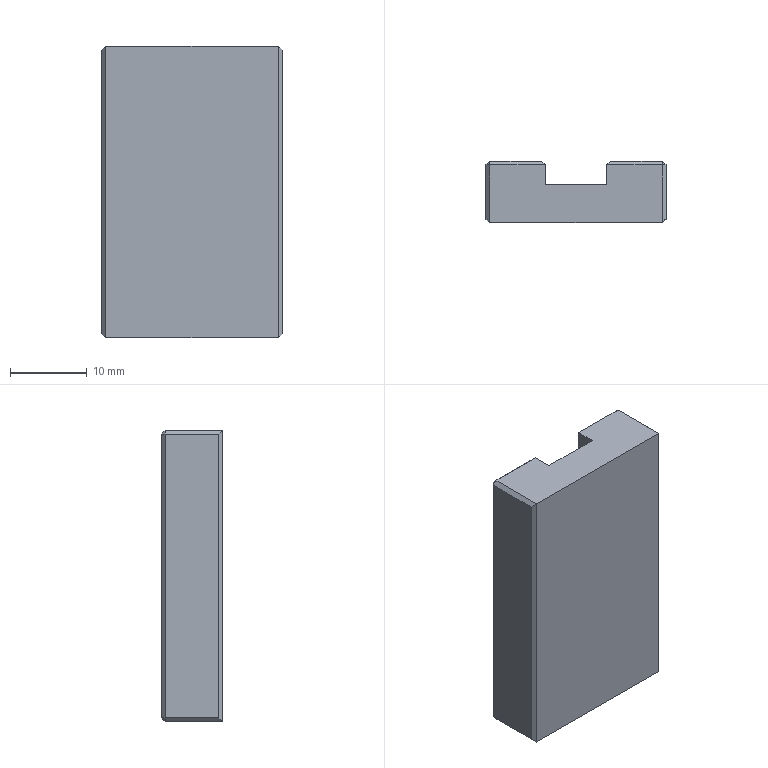Part | SolidWorks | features Chamfer 1, Extrusion 1 | 1 solid | 28 faces | box 23.5 x 8 x 38 mm | volume 6196 mm3 | plane 28
STEP:
#1=CARTESIAN_POINT('',(11.75,3.5,37.5));
#2=VERTEX_POINT('',#1);
#3=CARTESIAN_POINT('',(11.75,-3.5,37.5));
#4=VERTEX_POINT('',#3);
#5=CARTESIAN_POINT('',(11.75,-4.,37.5));
#6=DIRECTION('',(0.,-1.,0.));
#7=VECTOR('',#6,1000.);
#8=LINE('',#5,#7);
#9=EDGE_CURVE('',#2,#4,#8,.T.);
#10=ORIENTED_EDGE('',*,*,#9,.T.);
#11=CARTESIAN_POINT('',(11.75,-3.5,0.5));
#12=VERTEX_POINT('',#11);
#13=CARTESIAN_POINT('',(11.75,-3.5,38.));
#14=DIRECTION('',(0.,0.,-1.));
#15=VECTOR('',#14,1000.);
#16=LINE('',#13,#15);
#17=EDGE_CURVE('',#4,#12,#16,.T.);
#18=ORIENTED_EDGE('',*,*,#17,.T.);
#19=CARTESIAN_POINT('',(11.75,3.5,0.5));
#20=VERTEX_POINT('',#19);
#21=CARTESIAN_POINT('',(11.75,4.,0.5));
#22=DIRECTION('',(0.,1.,0.));
#23=VECTOR('',#22,1000.);
#24=LINE('',#21,#23);
#25=EDGE_CURVE('',#12,#20,#24,.T.);
#26=ORIENTED_EDGE('',*,*,#25,.T.);
#27=CARTESIAN_POINT('',(11.75,3.5,38.));
#28=DIRECTION('',(0.,0.,1.));
#29=VECTOR('',#28,1000.);
#30=LINE('',#27,#29);
#31=EDGE_CURVE('',#20,#2,#30,.T.);
#32=ORIENTED_EDGE('',*,*,#31,.T.);
#33=EDGE_LOOP('',(#10,#18,#26,#32));
#34=FACE_OUTER_BOUND('',#33,.T.);
#35=CARTESIAN_POINT('',(11.75,4.,38.));
#36=DIRECTION('',(-1.,0.,0.));
#37=DIRECTION('',(0.,-1.,0.));
#38=AXIS2_PLACEMENT_3D('',#35,#36,#37);
#39=PLANE('',#38);
#40=ADVANCED_FACE('',(#34),#39,.F.);
#41=CARTESIAN_POINT('',(4.5,4.,37.5));
#42=VERTEX_POINT('',#41);
#43=CARTESIAN_POINT('',(11.25,4.,37.5));
#44=VERTEX_POINT('',#43);
#45=CARTESIAN_POINT('',(11.75,4.,37.5));
#46=DIRECTION('',(1.,0.,0.));
#47=VECTOR('',#46,1000.);
#48=LINE('',#45,#47);
#49=EDGE_CURVE('',#42,#44,#48,.T.);
#50=ORIENTED_EDGE('',*,*,#49,.T.);
#51=CARTESIAN_POINT('',(11.25,4.,0.5));
#52=VERTEX_POINT('',#51);
#53=CARTESIAN_POINT('',(11.25,4.,38.));
#54=DIRECTION('',(0.,0.,-1.));
#55=VECTOR('',#54,1000.);
#56=LINE('',#53,#55);
#57=EDGE_CURVE('',#44,#52,#56,.T.);
#58=ORIENTED_EDGE('',*,*,#57,.T.);
#59=CARTESIAN_POINT('',(4.5,4.,0.5));
#60=VERTEX_POINT('',#59);
#61=CARTESIAN_POINT('',(4.,4.,0.5));
#62=DIRECTION('',(-1.,0.,0.));
#63=VECTOR('',#62,1000.);
#64=LINE('',#61,#63);
#65=EDGE_CURVE('',#52,#60,#64,.T.);
#66=ORIENTED_EDGE('',*,*,#65,.T.);
#67=CARTESIAN_POINT('',(4.5,4.,38.));
#68=DIRECTION('',(0.,0.,1.));
#69=VECTOR('',#68,1000.);
#70=LINE('',#67,#69);
#71=EDGE_CURVE('',#60,#42,#70,.T.);
#72=ORIENTED_EDGE('',*,*,#71,.T.);
#73=EDGE_LOOP('',(#50,#58,#66,#72));
#74=FACE_OUTER_BOUND('',#73,.T.);
#75=CARTESIAN_POINT('',(4.,4.,38.));
#76=DIRECTION('',(0.,-1.,0.));
#77=DIRECTION('',(1.,0.,0.));
#78=AXIS2_PLACEMENT_3D('',#75,#76,#77);
#79=PLANE('',#78);
#80=ADVANCED_FACE('',(#74),#79,.F.);
#81=CARTESIAN_POINT('',(4.,3.5,38.));
#82=VERTEX_POINT('',#81);
#83=CARTESIAN_POINT('',(4.,1.,38.));
#84=VERTEX_POINT('',#83);
#85=CARTESIAN_POINT('',(4.,1.,38.));
#86=DIRECTION('',(0.,-1.,0.));
#87=VECTOR('',#86,1000.);
#88=LINE('',#85,#87);
#89=EDGE_CURVE('',#82,#84,#88,.T.);
#90=ORIENTED_EDGE('',*,*,#89,.F.);
#91=CARTESIAN_POINT('',(4.,3.5,0.));
#92=VERTEX_POINT('',#91);
#93=CARTESIAN_POINT('',(4.,3.5,38.));
#94=DIRECTION('',(0.,0.,-1.));
#95=VECTOR('',#94,1000.);
#96=LINE('',#93,#95);
#97=EDGE_CURVE('',#82,#92,#96,.T.);
#98=ORIENTED_EDGE('',*,*,#97,.T.);
#99=CARTESIAN_POINT('',(4.,1.,0.));
#100=VERTEX_POINT('',#99);
#101=CARTESIAN_POINT('',(4.,1.,0.));
#102=DIRECTION('',(0.,-1.,0.));
#103=VECTOR('',#102,1000.);
#104=LINE('',#101,#103);
#105=EDGE_CURVE('',#92,#100,#104,.T.);
#106=ORIENTED_EDGE('',*,*,#105,.T.);
#107=CARTESIAN_POINT('',(4.,1.,38.));
#108=DIRECTION('',(0.,0.,-1.));
#109=VECTOR('',#108,1000.);
#110=LINE('',#107,#109);
#111=EDGE_CURVE('',#84,#100,#110,.T.);
#112=ORIENTED_EDGE('',*,*,#111,.F.);
#113=EDGE_LOOP('',(#90,#98,#106,#112));
#114=FACE_OUTER_BOUND('',#113,.T.);
#115=CARTESIAN_POINT('',(4.,1.,38.));
#116=DIRECTION('',(1.,0.,0.));
#117=DIRECTION('',(0.,1.,0.));
#118=AXIS2_PLACEMENT_3D('',#115,#116,#117);
#119=PLANE('',#118);
#120=ADVANCED_FACE('',(#114),#119,.F.);
#121=CARTESIAN_POINT('',(-4.,1.,0.));
#122=VERTEX_POINT('',#121);
#123=CARTESIAN_POINT('',(-4.,1.,0.));
#124=DIRECTION('',(-1.,0.,0.));
#125=VECTOR('',#124,1000.);
#126=LINE('',#123,#125);
#127=EDGE_CURVE('',#100,#122,#126,.T.);
#128=ORIENTED_EDGE('',*,*,#127,.T.);
#129=CARTESIAN_POINT('',(-4.,1.,38.));
#130=VERTEX_POINT('',#129);
#131=CARTESIAN_POINT('',(-4.,1.,38.));
#132=DIRECTION('',(0.,0.,-1.));
#133=VECTOR('',#132,1000.);
#134=LINE('',#131,#133);
#135=EDGE_CURVE('',#130,#122,#134,.T.);
#136=ORIENTED_EDGE('',*,*,#135,.F.);
#137=CARTESIAN_POINT('',(-4.,1.,38.));
#138=DIRECTION('',(-1.,0.,0.));
#139=VECTOR('',#138,1000.);
#140=LINE('',#137,#139);
#141=EDGE_CURVE('',#84,#130,#140,.T.);
#142=ORIENTED_EDGE('',*,*,#141,.F.);
#143=ORIENTED_EDGE('',*,*,#111,.T.);
#144=EDGE_LOOP('',(#128,#136,#142,#143));
#145=FACE_OUTER_BOUND('',#144,.T.);
#146=CARTESIAN_POINT('',(-4.,1.,38.));
#147=DIRECTION('',(0.,-1.,0.));
#148=DIRECTION('',(1.,0.,0.));
#149=AXIS2_PLACEMENT_3D('',#146,#147,#148);
#150=PLANE('',#149);
#151=ADVANCED_FACE('',(#145),#150,.F.);
#152=CARTESIAN_POINT('',(-4.,3.5,0.));
#153=VERTEX_POINT('',#152);
#154=CARTESIAN_POINT('',(-4.,4.,0.));
#155=DIRECTION('',(0.,1.,0.));
#156=VECTOR('',#155,1000.);
#157=LINE('',#154,#156);
#158=EDGE_CURVE('',#122,#153,#157,.T.);
#159=ORIENTED_EDGE('',*,*,#158,.T.);
#160=CARTESIAN_POINT('',(-4.,3.5,38.));
#161=VERTEX_POINT('',#160);
#162=CARTESIAN_POINT('',(-4.,3.5,38.));
#163=DIRECTION('',(0.,0.,1.));
#164=VECTOR('',#163,1000.);
#165=LINE('',#162,#164);
#166=EDGE_CURVE('',#153,#161,#165,.T.);
#167=ORIENTED_EDGE('',*,*,#166,.T.);
#168=CARTESIAN_POINT('',(-4.,4.,38.));
#169=DIRECTION('',(0.,1.,0.));
#170=VECTOR('',#169,1000.);
#171=LINE('',#168,#170);
#172=EDGE_CURVE('',#130,#161,#171,.T.);
#173=ORIENTED_EDGE('',*,*,#172,.F.);
#174=ORIENTED_EDGE('',*,*,#135,.T.);
#175=EDGE_LOOP('',(#159,#167,#173,#174));
#176=FACE_OUTER_BOUND('',#175,.T.);
#177=CARTESIAN_POINT('',(-4.,4.,38.));
#178=DIRECTION('',(-1.,0.,0.));
#179=DIRECTION('',(0.,0.,1.));
#180=AXIS2_PLACEMENT_3D('',#177,#178,#179);
#181=PLANE('',#180);
#182=ADVANCED_FACE('',(#176),#181,.F.);
#183=CARTESIAN_POINT('',(-11.25,4.,37.5));
#184=VERTEX_POINT('',#183);
#185=CARTESIAN_POINT('',(-4.5,4.,37.5));
#186=VERTEX_POINT('',#185);
#187=CARTESIAN_POINT('',(-4.,4.,37.5));
#188=DIRECTION('',(1.,0.,0.));
#189=VECTOR('',#188,1000.);
#190=LINE('',#187,#189);
#191=EDGE_CURVE('',#184,#186,#190,.T.);
#192=ORIENTED_EDGE('',*,*,#191,.T.);
#193=CARTESIAN_POINT('',(-4.5,4.,0.5));
#194=VERTEX_POINT('',#193);
#195=CARTESIAN_POINT('',(-4.5,4.,38.));
#196=DIRECTION('',(0.,0.,-1.));
#197=VECTOR('',#196,1000.);
#198=LINE('',#195,#197);
#199=EDGE_CURVE('',#186,#194,#198,.T.);
#200=ORIENTED_EDGE('',*,*,#199,.T.);
#201=CARTESIAN_POINT('',(-11.25,4.,0.5));
#202=VERTEX_POINT('',#201);
#203=CARTESIAN_POINT('',(-11.75,4.,0.5));
#204=DIRECTION('',(-1.,0.,0.));
#205=VECTOR('',#204,1000.);
#206=LINE('',#203,#205);
#207=EDGE_CURVE('',#194,#202,#206,.T.);
#208=ORIENTED_EDGE('',*,*,#207,.T.);
#209=CARTESIAN_POINT('',(-11.25,4.,38.));
#210=DIRECTION('',(0.,0.,1.));
#211=VECTOR('',#210,1000.);
#212=LINE('',#209,#211);
#213=EDGE_CURVE('',#202,#184,#212,.T.);
#214=ORIENTED_EDGE('',*,*,#213,.T.);
#215=EDGE_LOOP('',(#192,#200,#208,#214));
#216=FACE_OUTER_BOUND('',#215,.T.);
#217=CARTESIAN_POINT('',(-11.75,4.,38.));
#218=DIRECTION('',(0.,-1.,0.));
#219=DIRECTION('',(0.,0.,-1.));
#220=AXIS2_PLACEMENT_3D('',#217,#218,#219);
#221=PLANE('',#220);
#222=ADVANCED_FACE('',(#216),#221,.F.);
#223=CARTESIAN_POINT('',(-11.75,-3.5,0.5));
#224=VERTEX_POINT('',#223);
#225=CARTESIAN_POINT('',(-11.75,-3.5,37.5));
#226=VERTEX_POINT('',#225);
#227=CARTESIAN_POINT('',(-11.75,-3.5,38.));
#228=DIRECTION('',(0.,0.,1.));
#229=VECTOR('',#228,1000.);
#230=LINE('',#227,#229);
#231=EDGE_CURVE('',#224,#226,#230,.T.);
#232=ORIENTED_EDGE('',*,*,#231,.T.);
#233=CARTESIAN_POINT('',(-11.75,3.5,37.5));
#234=VERTEX_POINT('',#233);
#235=CARTESIAN_POINT('',(-11.75,4.,37.5));
#236=DIRECTION('',(0.,1.,0.));
#237=VECTOR('',#236,1000.);
#238=LINE('',#235,#237);
#239=EDGE_CURVE('',#226,#234,#238,.T.);
#240=ORIENTED_EDGE('',*,*,#239,.T.);
#241=CARTESIAN_POINT('',(-11.75,3.5,0.5));
#242=VERTEX_POINT('',#241);
#243=CARTESIAN_POINT('',(-11.75,3.5,38.));
#244=DIRECTION('',(0.,0.,-1.));
#245=VECTOR('',#244,1000.);
#246=LINE('',#243,#245);
#247=EDGE_CURVE('',#234,#242,#246,.T.);
#248=ORIENTED_EDGE('',*,*,#247,.T.);
#249=CARTESIAN_POINT('',(-11.75,4.,0.5));
#250=DIRECTION('',(0.,-1.,0.));
#251=VECTOR('',#250,1000.);
#252=LINE('',#249,#251);
#253=EDGE_CURVE('',#242,#224,#252,.T.);
#254=ORIENTED_EDGE('',*,*,#253,.T.);
#255=EDGE_LOOP('',(#232,#240,#248,#254));
#256=FACE_OUTER_BOUND('',#255,.T.);
#257=CARTESIAN_POINT('',(-11.75,4.,38.));
#258=DIRECTION('',(1.,0.,0.));
#259=DIRECTION('',(0.,1.,0.));
#260=AXIS2_PLACEMENT_3D('',#257,#258,#259);
#261=PLANE('',#260);
#262=ADVANCED_FACE('',(#256),#261,.F.);
#263=CARTESIAN_POINT('',(-11.25,-4.,0.));
#264=VERTEX_POINT('',#263);
#265=CARTESIAN_POINT('',(11.25,-4.,0.));
#266=VERTEX_POINT('',#265);
#267=CARTESIAN_POINT('',(-11.75,-4.,0.));
#268=DIRECTION('',(1.,0.,0.));
#269=VECTOR('',#268,1000.);
#270=LINE('',#267,#269);
#271=EDGE_CURVE('',#264,#266,#270,.T.);
#272=ORIENTED_EDGE('',*,*,#271,.T.);
#273=CARTESIAN_POINT('',(11.25,-4.,38.));
#274=VERTEX_POINT('',#273);
#275=CARTESIAN_POINT('',(11.25,-4.,38.));
#276=DIRECTION('',(0.,0.,1.));
#277=VECTOR('',#276,1000.);
#278=LINE('',#275,#277);
#279=EDGE_CURVE('',#266,#274,#278,.T.);
#280=ORIENTED_EDGE('',*,*,#279,.T.);
#281=CARTESIAN_POINT('',(-11.25,-4.,38.));
#282=VERTEX_POINT('',#281);
#283=CARTESIAN_POINT('',(-11.75,-4.,38.));
#284=DIRECTION('',(1.,0.,0.));
#285=VECTOR('',#284,1000.);
#286=LINE('',#283,#285);
#287=EDGE_CURVE('',#282,#274,#286,.T.);
#288=ORIENTED_EDGE('',*,*,#287,.F.);
#289=CARTESIAN_POINT('',(-11.25,-4.,38.));
#290=DIRECTION('',(0.,0.,-1.));
#291=VECTOR('',#290,1000.);
#292=LINE('',#289,#291);
#293=EDGE_CURVE('',#282,#264,#292,.T.);
#294=ORIENTED_EDGE('',*,*,#293,.T.);
#295=EDGE_LOOP('',(#272,#280,#288,#294));
#296=FACE_OUTER_BOUND('',#295,.T.);
#297=CARTESIAN_POINT('',(-11.75,-4.,38.));
#298=DIRECTION('',(0.,1.,0.));
#299=DIRECTION('',(0.,0.,1.));
#300=AXIS2_PLACEMENT_3D('',#297,#298,#299);
#301=PLANE('',#300);
#302=ADVANCED_FACE('',(#296),#301,.F.);
#303=ORIENTED_EDGE('',*,*,#287,.T.);
#304=CARTESIAN_POINT('',(11.25,3.5,38.));
#305=VERTEX_POINT('',#304);
#306=CARTESIAN_POINT('',(11.25,4.,38.));
#307=DIRECTION('',(0.,1.,0.));
#308=VECTOR('',#307,1000.);
#309=LINE('',#306,#308);
#310=EDGE_CURVE('',#274,#305,#309,.T.);
#311=ORIENTED_EDGE('',*,*,#310,.T.);
#312=CARTESIAN_POINT('',(4.,3.5,38.));
#313=DIRECTION('',(-1.,0.,0.));
#314=VECTOR('',#313,1000.);
#315=LINE('',#312,#314);
#316=EDGE_CURVE('',#305,#82,#315,.T.);
#317=ORIENTED_EDGE('',*,*,#316,.T.);
#318=ORIENTED_EDGE('',*,*,#89,.T.);
#319=ORIENTED_EDGE('',*,*,#141,.T.);
#320=ORIENTED_EDGE('',*,*,#172,.T.);
#321=CARTESIAN_POINT('',(-11.25,3.5,38.));
#322=VERTEX_POINT('',#321);
#323=CARTESIAN_POINT('',(-11.75,3.5,38.));
#324=DIRECTION('',(-1.,0.,0.));
#325=VECTOR('',#324,1000.);
#326=LINE('',#323,#325);
#327=EDGE_CURVE('',#161,#322,#326,.T.);
#328=ORIENTED_EDGE('',*,*,#327,.T.);
#329=CARTESIAN_POINT('',(-11.25,-4.,38.));
#330=DIRECTION('',(0.,-1.,0.));
#331=VECTOR('',#330,1000.);
#332=LINE('',#329,#331);
#333=EDGE_CURVE('',#322,#282,#332,.T.);
#334=ORIENTED_EDGE('',*,*,#333,.T.);
#335=EDGE_LOOP('',(#303,#311,#317,#318,#319,#320,#328,#334));
#336=FACE_OUTER_BOUND('',#335,.T.);
#337=CARTESIAN_POINT('',(0.,0.,38.));
#338=DIRECTION('',(0.,0.,1.));
#339=DIRECTION('',(1.,0.,0.));
#340=AXIS2_PLACEMENT_3D('',#337,#338,#339);
#341=PLANE('',#340);
#342=ADVANCED_FACE('',(#336),#341,.T.);
#343=CARTESIAN_POINT('',(11.25,3.5,0.));
#344=VERTEX_POINT('',#343);
#345=CARTESIAN_POINT('',(0.,3.5,0.));
#346=DIRECTION('',(1.,0.,0.));
#347=VECTOR('',#346,1000.);
#348=LINE('',#345,#347);
#349=EDGE_CURVE('',#92,#344,#348,.T.);
#350=ORIENTED_EDGE('',*,*,#349,.T.);
#351=CARTESIAN_POINT('',(11.25,0.,0.));
#352=DIRECTION('',(0.,-1.,0.));
#353=VECTOR('',#352,1000.);
#354=LINE('',#351,#353);
#355=EDGE_CURVE('',#344,#266,#354,.T.);
#356=ORIENTED_EDGE('',*,*,#355,.T.);
#357=ORIENTED_EDGE('',*,*,#271,.F.);
#358=CARTESIAN_POINT('',(-11.25,3.5,0.));
#359=VERTEX_POINT('',#358);
#360=CARTESIAN_POINT('',(-11.25,0.,0.));
#361=DIRECTION('',(0.,1.,0.));
#362=VECTOR('',#361,1000.);
#363=LINE('',#360,#362);
#364=EDGE_CURVE('',#264,#359,#363,.T.);
#365=ORIENTED_EDGE('',*,*,#364,.T.);
#366=CARTESIAN_POINT('',(0.,3.5,0.));
#367=DIRECTION('',(1.,0.,0.));
#368=VECTOR('',#367,1000.);
#369=LINE('',#366,#368);
#370=EDGE_CURVE('',#359,#153,#369,.T.);
#371=ORIENTED_EDGE('',*,*,#370,.T.);
#372=ORIENTED_EDGE('',*,*,#158,.F.);
#373=ORIENTED_EDGE('',*,*,#127,.F.);
#374=ORIENTED_EDGE('',*,*,#105,.F.);
#375=EDGE_LOOP('',(#350,#356,#357,#365,#371,#372,#373,#374));
#376=FACE_OUTER_BOUND('',#375,.T.);
#377=CARTESIAN_POINT('',(0.,0.,0.));
#378=DIRECTION('',(0.,0.,1.));
#379=DIRECTION('',(1.,0.,0.));
#380=AXIS2_PLACEMENT_3D('',#377,#378,#379);
#381=PLANE('',#380);
#382=ADVANCED_FACE('',(#376),#381,.F.);
#383=CARTESIAN_POINT('',(4.333,3.833,0.3333));
#384=DIRECTION('',(0.5774,0.5774,0.5774));
#385=VECTOR('',#384,1000.);
#386=LINE('',#383,#385);
#387=EDGE_CURVE('',#92,#60,#386,.T.);
#388=ORIENTED_EDGE('',*,*,#387,.F.);
#389=ORIENTED_EDGE('',*,*,#97,.F.);
#390=CARTESIAN_POINT('',(4.,3.5,38.));
#391=DIRECTION('',(-0.5774,-0.5774,0.5774));
#392=VECTOR('',#391,1000.);
#393=LINE('',#390,#392);
#394=EDGE_CURVE('',#42,#82,#393,.T.);
#395=ORIENTED_EDGE('',*,*,#394,.F.);
#396=ORIENTED_EDGE('',*,*,#71,.F.);
#397=EDGE_LOOP('',(#388,#389,#395,#396));
#398=FACE_OUTER_BOUND('',#397,.T.);
#399=CARTESIAN_POINT('',(4.,3.5,38.));
#400=DIRECTION('',(0.7071,-0.7071,0.));
#401=DIRECTION('',(0.,0.,-1.));
#402=AXIS2_PLACEMENT_3D('',#399,#400,#401);
#403=PLANE('',#402);
#404=ADVANCED_FACE('',(#398),#403,.F.);
#405=ORIENTED_EDGE('',*,*,#394,.T.);
#406=ORIENTED_EDGE('',*,*,#316,.F.);
#407=CARTESIAN_POINT('',(11.25,3.5,38.));
#408=DIRECTION('',(0.,-0.7071,0.7071));
#409=VECTOR('',#408,1000.);
#410=LINE('',#407,#409);
#411=EDGE_CURVE('',#44,#305,#410,.T.);
#412=ORIENTED_EDGE('',*,*,#411,.F.);
#413=ORIENTED_EDGE('',*,*,#49,.F.);
#414=EDGE_LOOP('',(#405,#406,#412,#413));
#415=FACE_OUTER_BOUND('',#414,.T.);
#416=CARTESIAN_POINT('',(0.,3.5,38.));
#417=DIRECTION('',(0.,0.7071,0.7071));
#418=DIRECTION('',(1.,0.,0.));
#419=AXIS2_PLACEMENT_3D('',#416,#417,#418);
#420=PLANE('',#419);
#421=ADVANCED_FACE('',(#415),#420,.T.);
#422=CARTESIAN_POINT('',(11.75,3.5,0.5));
#423=DIRECTION('',(0.7071,-0.7071,0.));
#424=VECTOR('',#423,1000.);
#425=LINE('',#422,#424);
#426=EDGE_CURVE('',#52,#20,#425,.T.);
#427=ORIENTED_EDGE('',*,*,#426,.F.);
#428=ORIENTED_EDGE('',*,*,#57,.F.);
#429=CARTESIAN_POINT('',(11.5,3.75,37.5));
#430=DIRECTION('',(-0.7071,0.7071,0.));
#431=VECTOR('',#430,1000.);
#432=LINE('',#429,#431);
#433=EDGE_CURVE('',#2,#44,#432,.T.);
#434=ORIENTED_EDGE('',*,*,#433,.F.);
#435=ORIENTED_EDGE('',*,*,#31,.F.);
#436=EDGE_LOOP('',(#427,#428,#434,#435));
#437=FACE_OUTER_BOUND('',#436,.T.);
#438=CARTESIAN_POINT('',(11.25,4.,38.));
#439=DIRECTION('',(-0.7071,-0.7071,0.));
#440=DIRECTION('',(0.,0.,-1.));
#441=AXIS2_PLACEMENT_3D('',#438,#439,#440);
#442=PLANE('',#441);
#443=ADVANCED_FACE('',(#437),#442,.F.);
#444=ORIENTED_EDGE('',*,*,#387,.T.);
#445=ORIENTED_EDGE('',*,*,#65,.F.);
#446=CARTESIAN_POINT('',(11.25,3.75,0.25));
#447=DIRECTION('',(0.,0.7071,0.7071));
#448=VECTOR('',#447,1000.);
#449=LINE('',#446,#448);
#450=EDGE_CURVE('',#344,#52,#449,.T.);
#451=ORIENTED_EDGE('',*,*,#450,.F.);
#452=ORIENTED_EDGE('',*,*,#349,.F.);
#453=EDGE_LOOP('',(#444,#445,#451,#452));
#454=FACE_OUTER_BOUND('',#453,.T.);
#455=CARTESIAN_POINT('',(4.,4.,0.5));
#456=DIRECTION('',(0.,-0.7071,0.7071));
#457=DIRECTION('',(-1.,0.,0.));
#458=AXIS2_PLACEMENT_3D('',#455,#456,#457);
#459=PLANE('',#458);
#460=ADVANCED_FACE('',(#454),#459,.F.);
#461=ORIENTED_EDGE('',*,*,#433,.T.);
#462=ORIENTED_EDGE('',*,*,#411,.T.);
#463=CARTESIAN_POINT('',(11.25,3.5,38.));
#464=DIRECTION('',(-0.7071,0.,0.7071));
#465=VECTOR('',#464,1000.);
#466=LINE('',#463,#465);
#467=EDGE_CURVE('',#2,#305,#466,.T.);
#468=ORIENTED_EDGE('',*,*,#467,.F.);
#469=EDGE_LOOP('',(#461,#462,#468));
#470=FACE_OUTER_BOUND('',#469,.T.);
#471=CARTESIAN_POINT('',(11.25,3.5,38.));
#472=DIRECTION('',(0.5774,0.5774,0.5774));
#473=DIRECTION('',(0.7071,0.,-0.7071));
#474=AXIS2_PLACEMENT_3D('',#471,#472,#473);
#475=PLANE('',#474);
#476=ADVANCED_FACE('',(#470),#475,.T.);
#477=ORIENTED_EDGE('',*,*,#450,.T.);
#478=ORIENTED_EDGE('',*,*,#426,.T.);
#479=CARTESIAN_POINT('',(11.75,3.5,0.5));
#480=DIRECTION('',(0.7071,0.,0.7071));
#481=VECTOR('',#480,1000.);
#482=LINE('',#479,#481);
#483=EDGE_CURVE('',#344,#20,#482,.T.);
#484=ORIENTED_EDGE('',*,*,#483,.F.);
#485=EDGE_LOOP('',(#477,#478,#484));
#486=FACE_OUTER_BOUND('',#485,.T.);
#487=CARTESIAN_POINT('',(11.75,3.5,0.5));
#488=DIRECTION('',(0.5774,0.5774,-0.5774));
#489=DIRECTION('',(-0.7071,0.,-0.7071));
#490=AXIS2_PLACEMENT_3D('',#487,#488,#489);
#491=PLANE('',#490);
#492=ADVANCED_FACE('',(#486),#491,.T.);
#493=ORIENTED_EDGE('',*,*,#467,.T.);
#494=ORIENTED_EDGE('',*,*,#310,.F.);
#495=CARTESIAN_POINT('',(12.583,-2.667,36.667));
#496=DIRECTION('',(-0.5774,-0.5774,0.5774));
#497=VECTOR('',#496,1000.);
#498=LINE('',#495,#497);
#499=EDGE_CURVE('',#4,#274,#498,.T.);
#500=ORIENTED_EDGE('',*,*,#499,.F.);
#501=ORIENTED_EDGE('',*,*,#9,.F.);
#502=EDGE_LOOP('',(#493,#494,#500,#501));
#503=FACE_OUTER_BOUND('',#502,.T.);
#504=CARTESIAN_POINT('',(11.25,0.,38.));
#505=DIRECTION('',(0.7071,0.,0.7071));
#506=DIRECTION('',(0.,-1.,0.));
#507=AXIS2_PLACEMENT_3D('',#504,#505,#506);
#508=PLANE('',#507);
#509=ADVANCED_FACE('',(#503),#508,.T.);
#510=ORIENTED_EDGE('',*,*,#483,.T.);
#511=ORIENTED_EDGE('',*,*,#25,.F.);
#512=CARTESIAN_POINT('',(14.25,-1.,3.));
#513=DIRECTION('',(0.5774,0.5774,0.5774));
#514=VECTOR('',#513,1000.);
#515=LINE('',#512,#514);
#516=EDGE_CURVE('',#266,#12,#515,.T.);
#517=ORIENTED_EDGE('',*,*,#516,.F.);
#518=ORIENTED_EDGE('',*,*,#355,.F.);
#519=EDGE_LOOP('',(#510,#511,#517,#518));
#520=FACE_OUTER_BOUND('',#519,.T.);
#521=CARTESIAN_POINT('',(11.75,4.,0.5));
#522=DIRECTION('',(-0.7071,0.,0.7071));
#523=DIRECTION('',(0.,1.,0.));
#524=AXIS2_PLACEMENT_3D('',#521,#522,#523);
#525=PLANE('',#524);
#526=ADVANCED_FACE('',(#520),#525,.F.);
#527=ORIENTED_EDGE('',*,*,#499,.T.);
#528=ORIENTED_EDGE('',*,*,#279,.F.);
#529=ORIENTED_EDGE('',*,*,#516,.T.);
#530=ORIENTED_EDGE('',*,*,#17,.F.);
#531=EDGE_LOOP('',(#527,#528,#529,#530));
#532=FACE_OUTER_BOUND('',#531,.T.);
#533=CARTESIAN_POINT('',(11.75,-3.5,38.));
#534=DIRECTION('',(-0.7071,0.7071,0.));
#535=DIRECTION('',(0.,0.,-1.));
#536=AXIS2_PLACEMENT_3D('',#533,#534,#535);
#537=PLANE('',#536);
#538=ADVANCED_FACE('',(#532),#537,.F.);
#539=CARTESIAN_POINT('',(-11.25,3.5,0.));
#540=DIRECTION('',(0.,-0.7071,-0.7071));
#541=VECTOR('',#540,1000.);
#542=LINE('',#539,#541);
#543=EDGE_CURVE('',#202,#359,#542,.T.);
#544=ORIENTED_EDGE('',*,*,#543,.F.);
#545=ORIENTED_EDGE('',*,*,#207,.F.);
#546=CARTESIAN_POINT('',(-6.917,6.417,2.917));
#547=DIRECTION('',(-0.5774,0.5774,0.5774));
#548=VECTOR('',#547,1000.);
#549=LINE('',#546,#548);
#550=EDGE_CURVE('',#153,#194,#549,.T.);
#551=ORIENTED_EDGE('',*,*,#550,.F.);
#552=ORIENTED_EDGE('',*,*,#370,.F.);
#553=EDGE_LOOP('',(#544,#545,#551,#552));
#554=FACE_OUTER_BOUND('',#553,.T.);
#555=CARTESIAN_POINT('',(-11.75,4.,0.5));
#556=DIRECTION('',(0.,-0.7071,0.7071));
#557=DIRECTION('',(-1.,0.,0.));
#558=AXIS2_PLACEMENT_3D('',#555,#556,#557);
#559=PLANE('',#558);
#560=ADVANCED_FACE('',(#554),#559,.F.);
#561=ORIENTED_EDGE('',*,*,#550,.T.);
#562=ORIENTED_EDGE('',*,*,#199,.F.);
#563=CARTESIAN_POINT('',(-2.667,2.167,39.333));
#564=DIRECTION('',(-0.5774,0.5774,-0.5774));
#565=VECTOR('',#564,1000.);
#566=LINE('',#563,#565);
#567=EDGE_CURVE('',#161,#186,#566,.T.);
#568=ORIENTED_EDGE('',*,*,#567,.F.);
#569=ORIENTED_EDGE('',*,*,#166,.F.);
#570=EDGE_LOOP('',(#561,#562,#568,#569));
#571=FACE_OUTER_BOUND('',#570,.T.);
#572=CARTESIAN_POINT('',(-4.5,4.,38.));
#573=DIRECTION('',(-0.7071,-0.7071,0.));
#574=DIRECTION('',(0.,0.,-1.));
#575=AXIS2_PLACEMENT_3D('',#572,#573,#574);
#576=PLANE('',#575);
#577=ADVANCED_FACE('',(#571),#576,.F.);
#578=CARTESIAN_POINT('',(-11.25,3.5,0.));
#579=DIRECTION('',(0.7071,0.,-0.7071));
#580=VECTOR('',#579,1000.);
#581=LINE('',#578,#580);
#582=EDGE_CURVE('',#242,#359,#581,.T.);
#583=ORIENTED_EDGE('',*,*,#582,.F.);
#584=CARTESIAN_POINT('',(-11.5,3.75,0.5));
#585=DIRECTION('',(-0.7071,-0.7071,0.));
#586=VECTOR('',#585,1000.);
#587=LINE('',#584,#586);
#588=EDGE_CURVE('',#202,#242,#587,.T.);
#589=ORIENTED_EDGE('',*,*,#588,.F.);
#590=ORIENTED_EDGE('',*,*,#543,.T.);
#591=EDGE_LOOP('',(#583,#589,#590));
#592=FACE_OUTER_BOUND('',#591,.T.);
#593=CARTESIAN_POINT('',(-11.25,3.5,0.));
#594=DIRECTION('',(-0.5774,0.5774,-0.5774));
#595=DIRECTION('',(-0.7071,0.,0.7071));
#596=AXIS2_PLACEMENT_3D('',#593,#594,#595);
#597=PLANE('',#596);
#598=ADVANCED_FACE('',(#592),#597,.T.);
#599=ORIENTED_EDGE('',*,*,#588,.T.);
#600=ORIENTED_EDGE('',*,*,#247,.F.);
#601=CARTESIAN_POINT('',(-11.75,3.5,37.5));
#602=DIRECTION('',(-0.7071,-0.7071,0.));
#603=VECTOR('',#602,1000.);
#604=LINE('',#601,#603);
#605=EDGE_CURVE('',#184,#234,#604,.T.);
#606=ORIENTED_EDGE('',*,*,#605,.F.);
#607=ORIENTED_EDGE('',*,*,#213,.F.);
#608=EDGE_LOOP('',(#599,#600,#606,#607));
#609=FACE_OUTER_BOUND('',#608,.T.);
#610=CARTESIAN_POINT('',(-11.75,3.5,38.));
#611=DIRECTION('',(0.7071,-0.7071,0.));
#612=DIRECTION('',(0.,0.,-1.));
#613=AXIS2_PLACEMENT_3D('',#610,#611,#612);
#614=PLANE('',#613);
#615=ADVANCED_FACE('',(#609),#614,.F.);
#616=ORIENTED_EDGE('',*,*,#567,.T.);
#617=ORIENTED_EDGE('',*,*,#191,.F.);
#618=CARTESIAN_POINT('',(-11.25,3.75,37.75));
#619=DIRECTION('',(0.,0.7071,-0.7071));
#620=VECTOR('',#619,1000.);
#621=LINE('',#618,#620);
#622=EDGE_CURVE('',#322,#184,#621,.T.);
#623=ORIENTED_EDGE('',*,*,#622,.F.);
#624=ORIENTED_EDGE('',*,*,#327,.F.);
#625=EDGE_LOOP('',(#616,#617,#623,#624));
#626=FACE_OUTER_BOUND('',#625,.T.);
#627=CARTESIAN_POINT('',(0.,3.5,38.));
#628=DIRECTION('',(0.,0.7071,0.7071));
#629=DIRECTION('',(1.,0.,0.));
#630=AXIS2_PLACEMENT_3D('',#627,#628,#629);
#631=PLANE('',#630);
#632=ADVANCED_FACE('',(#626),#631,.T.);
#633=ORIENTED_EDGE('',*,*,#582,.T.);
#634=ORIENTED_EDGE('',*,*,#364,.F.);
#635=CARTESIAN_POINT('',(-14.25,-1.,3.));
#636=DIRECTION('',(0.5774,-0.5774,-0.5774));
#637=VECTOR('',#636,1000.);
#638=LINE('',#635,#637);
#639=EDGE_CURVE('',#224,#264,#638,.T.);
#640=ORIENTED_EDGE('',*,*,#639,.F.);
#641=ORIENTED_EDGE('',*,*,#253,.F.);
#642=EDGE_LOOP('',(#633,#634,#640,#641));
#643=FACE_OUTER_BOUND('',#642,.T.);
#644=CARTESIAN_POINT('',(-11.75,4.,0.5));
#645=DIRECTION('',(0.7071,0.,0.7071));
#646=DIRECTION('',(0.,-1.,0.));
#647=AXIS2_PLACEMENT_3D('',#644,#645,#646);
#648=PLANE('',#647);
#649=ADVANCED_FACE('',(#643),#648,.F.);
#650=ORIENTED_EDGE('',*,*,#622,.T.);
#651=ORIENTED_EDGE('',*,*,#605,.T.);
#652=CARTESIAN_POINT('',(-11.75,3.5,37.5));
#653=DIRECTION('',(-0.7071,0.,-0.7071));
#654=VECTOR('',#653,1000.);
#655=LINE('',#652,#654);
#656=EDGE_CURVE('',#322,#234,#655,.T.);
#657=ORIENTED_EDGE('',*,*,#656,.F.);
#658=EDGE_LOOP('',(#650,#651,#657));
#659=FACE_OUTER_BOUND('',#658,.T.);
#660=CARTESIAN_POINT('',(-11.75,3.5,37.5));
#661=DIRECTION('',(-0.5774,0.5774,0.5774));
#662=DIRECTION('',(0.7071,0.,0.7071));
#663=AXIS2_PLACEMENT_3D('',#660,#661,#662);
#664=PLANE('',#663);
#665=ADVANCED_FACE('',(#659),#664,.T.);
#666=ORIENTED_EDGE('',*,*,#639,.T.);
#667=ORIENTED_EDGE('',*,*,#293,.F.);
#668=CARTESIAN_POINT('',(-11.25,-4.,38.));
#669=DIRECTION('',(0.5774,-0.5774,0.5774));
#670=VECTOR('',#669,1000.);
#671=LINE('',#668,#670);
#672=EDGE_CURVE('',#226,#282,#671,.T.);
#673=ORIENTED_EDGE('',*,*,#672,.F.);
#674=ORIENTED_EDGE('',*,*,#231,.F.);
#675=EDGE_LOOP('',(#666,#667,#673,#674));
#676=FACE_OUTER_BOUND('',#675,.T.);
#677=CARTESIAN_POINT('',(-11.25,-4.,38.));
#678=DIRECTION('',(0.7071,0.7071,0.));
#679=DIRECTION('',(0.,0.,-1.));
#680=AXIS2_PLACEMENT_3D('',#677,#678,#679);
#681=PLANE('',#680);
#682=ADVANCED_FACE('',(#676),#681,.F.);
#683=ORIENTED_EDGE('',*,*,#656,.T.);
#684=ORIENTED_EDGE('',*,*,#239,.F.);
#685=ORIENTED_EDGE('',*,*,#672,.T.);
#686=ORIENTED_EDGE('',*,*,#333,.F.);
#687=EDGE_LOOP('',(#683,#684,#685,#686));
#688=FACE_OUTER_BOUND('',#687,.T.);
#689=CARTESIAN_POINT('',(-11.25,0.,38.));
#690=DIRECTION('',(-0.7071,0.,0.7071));
#691=DIRECTION('',(0.,1.,0.));
#692=AXIS2_PLACEMENT_3D('',#689,#690,#691);
#693=PLANE('',#692);
#694=ADVANCED_FACE('',(#688),#693,.T.);
#695=CLOSED_SHELL('',(#40,#80,#120,#151,#182,#222,#262,#302,#342,#382,#404,#421,#443,#460,#476,#492,#509,#526,#538,#560,#577,#598,#615,#632,#649,#665,#682,#694));
#696=MANIFOLD_SOLID_BREP('',#695);
#697=CARTESIAN_POINT('',(0.,0.,0.));
#698=DIRECTION('',(0.,0.,1.));
#699=DIRECTION('',(1.,0.,0.));
#700=AXIS2_PLACEMENT_3D('',#697,#698,#699);
#701=(LENGTH_UNIT()NAMED_UNIT(*)SI_UNIT(.MILLI.,.METRE.));
#702=UNCERTAINTY_MEASURE_WITH_UNIT(LENGTH_MEASURE(0.00001),#701,'','');
#703=(NAMED_UNIT(*)PLANE_ANGLE_UNIT()SI_UNIT($,.RADIAN.));
#704=(NAMED_UNIT(*)SI_UNIT($,.STERADIAN.)SOLID_ANGLE_UNIT());
#705=(GEOMETRIC_REPRESENTATION_CONTEXT(3)GLOBAL_UNCERTAINTY_ASSIGNED_CONTEXT((#702))GLOBAL_UNIT_ASSIGNED_CONTEXT((#701,#703,#704))REPRESENTATION_CONTEXT('',''));
#706=ADVANCED_BREP_SHAPE_REPRESENTATION('',(#696,#700),#705);